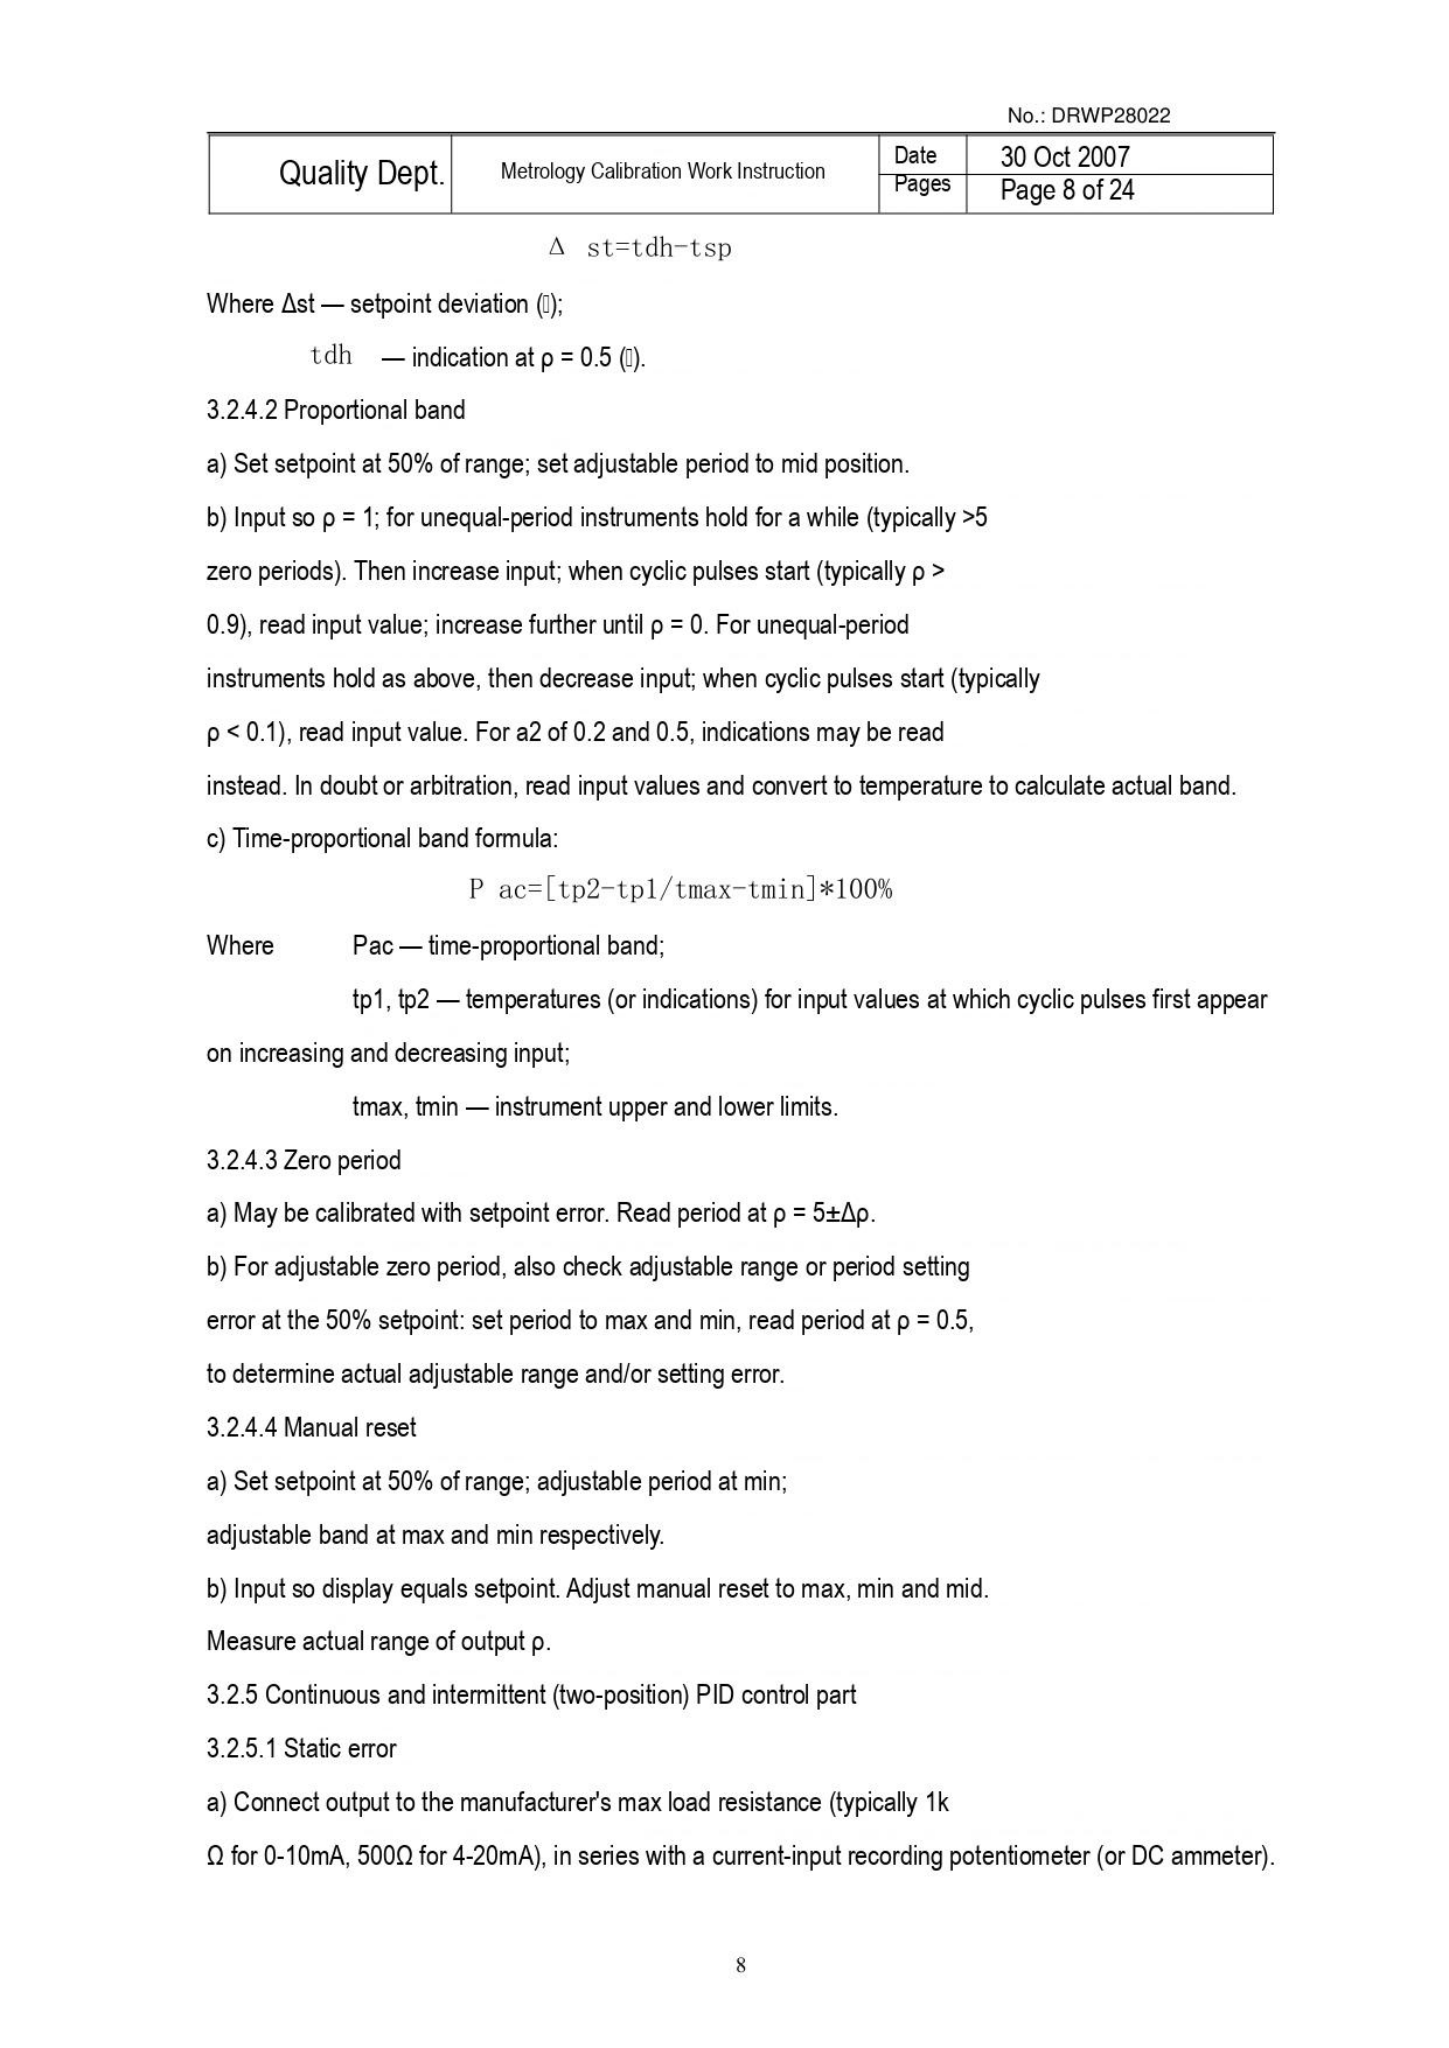No.: DRWP28022

| Quality Dept. | Metrology Calibration Work Instruction | Date | 30 Oct 2007 |
|---|---|---|---|
| | | Pages | Page 8 of 24 |

Δ st=tdh-tsp

Where Δst — setpoint deviation ();

tdh — indication at ρ = 0.5 ().

3.2.4.2 Proportional band

a) Set setpoint at 50% of range; set adjustable period to mid position.

b) Input so ρ = 1; for unequal-period instruments hold for a while (typically >5 zero periods). Then increase input; when cyclic pulses start (typically ρ > 0.9), read input value; increase further until ρ = 0. For unequal-period instruments hold as above, then decrease input; when cyclic pulses start (typically ρ < 0.1), read input value. For a2 of 0.2 and 0.5, indications may be read instead. In doubt or arbitration, read input values and convert to temperature to calculate actual band.

c) Time-proportional band formula:

P ac=[tp2-tp1/tmax-tmin]*100%

Where Pac — time-proportional band;

tp1, tp2 — temperatures (or indications) for input values at which cyclic pulses first appear on increasing and decreasing input;

tmax, tmin — instrument upper and lower limits.

3.2.4.3 Zero period

a) May be calibrated with setpoint error. Read period at ρ = 5±Δρ.

b) For adjustable zero period, also check adjustable range or period setting error at the 50% setpoint: set period to max and min, read period at ρ = 0.5, to determine actual adjustable range and/or setting error.

3.2.4.4 Manual reset

a) Set setpoint at 50% of range; adjustable period at min; adjustable band at max and min respectively.

b) Input so display equals setpoint. Adjust manual reset to max, min and mid. Measure actual range of output ρ.

3.2.5 Continuous and intermittent (two-position) PID control part

3.2.5.1 Static error

a) Connect output to the manufacturer's max load resistance (typically 1k Ω for 0-10mA, 500Ω for 4-20mA), in series with a current-input recording potentiometer (or DC ammeter).

8
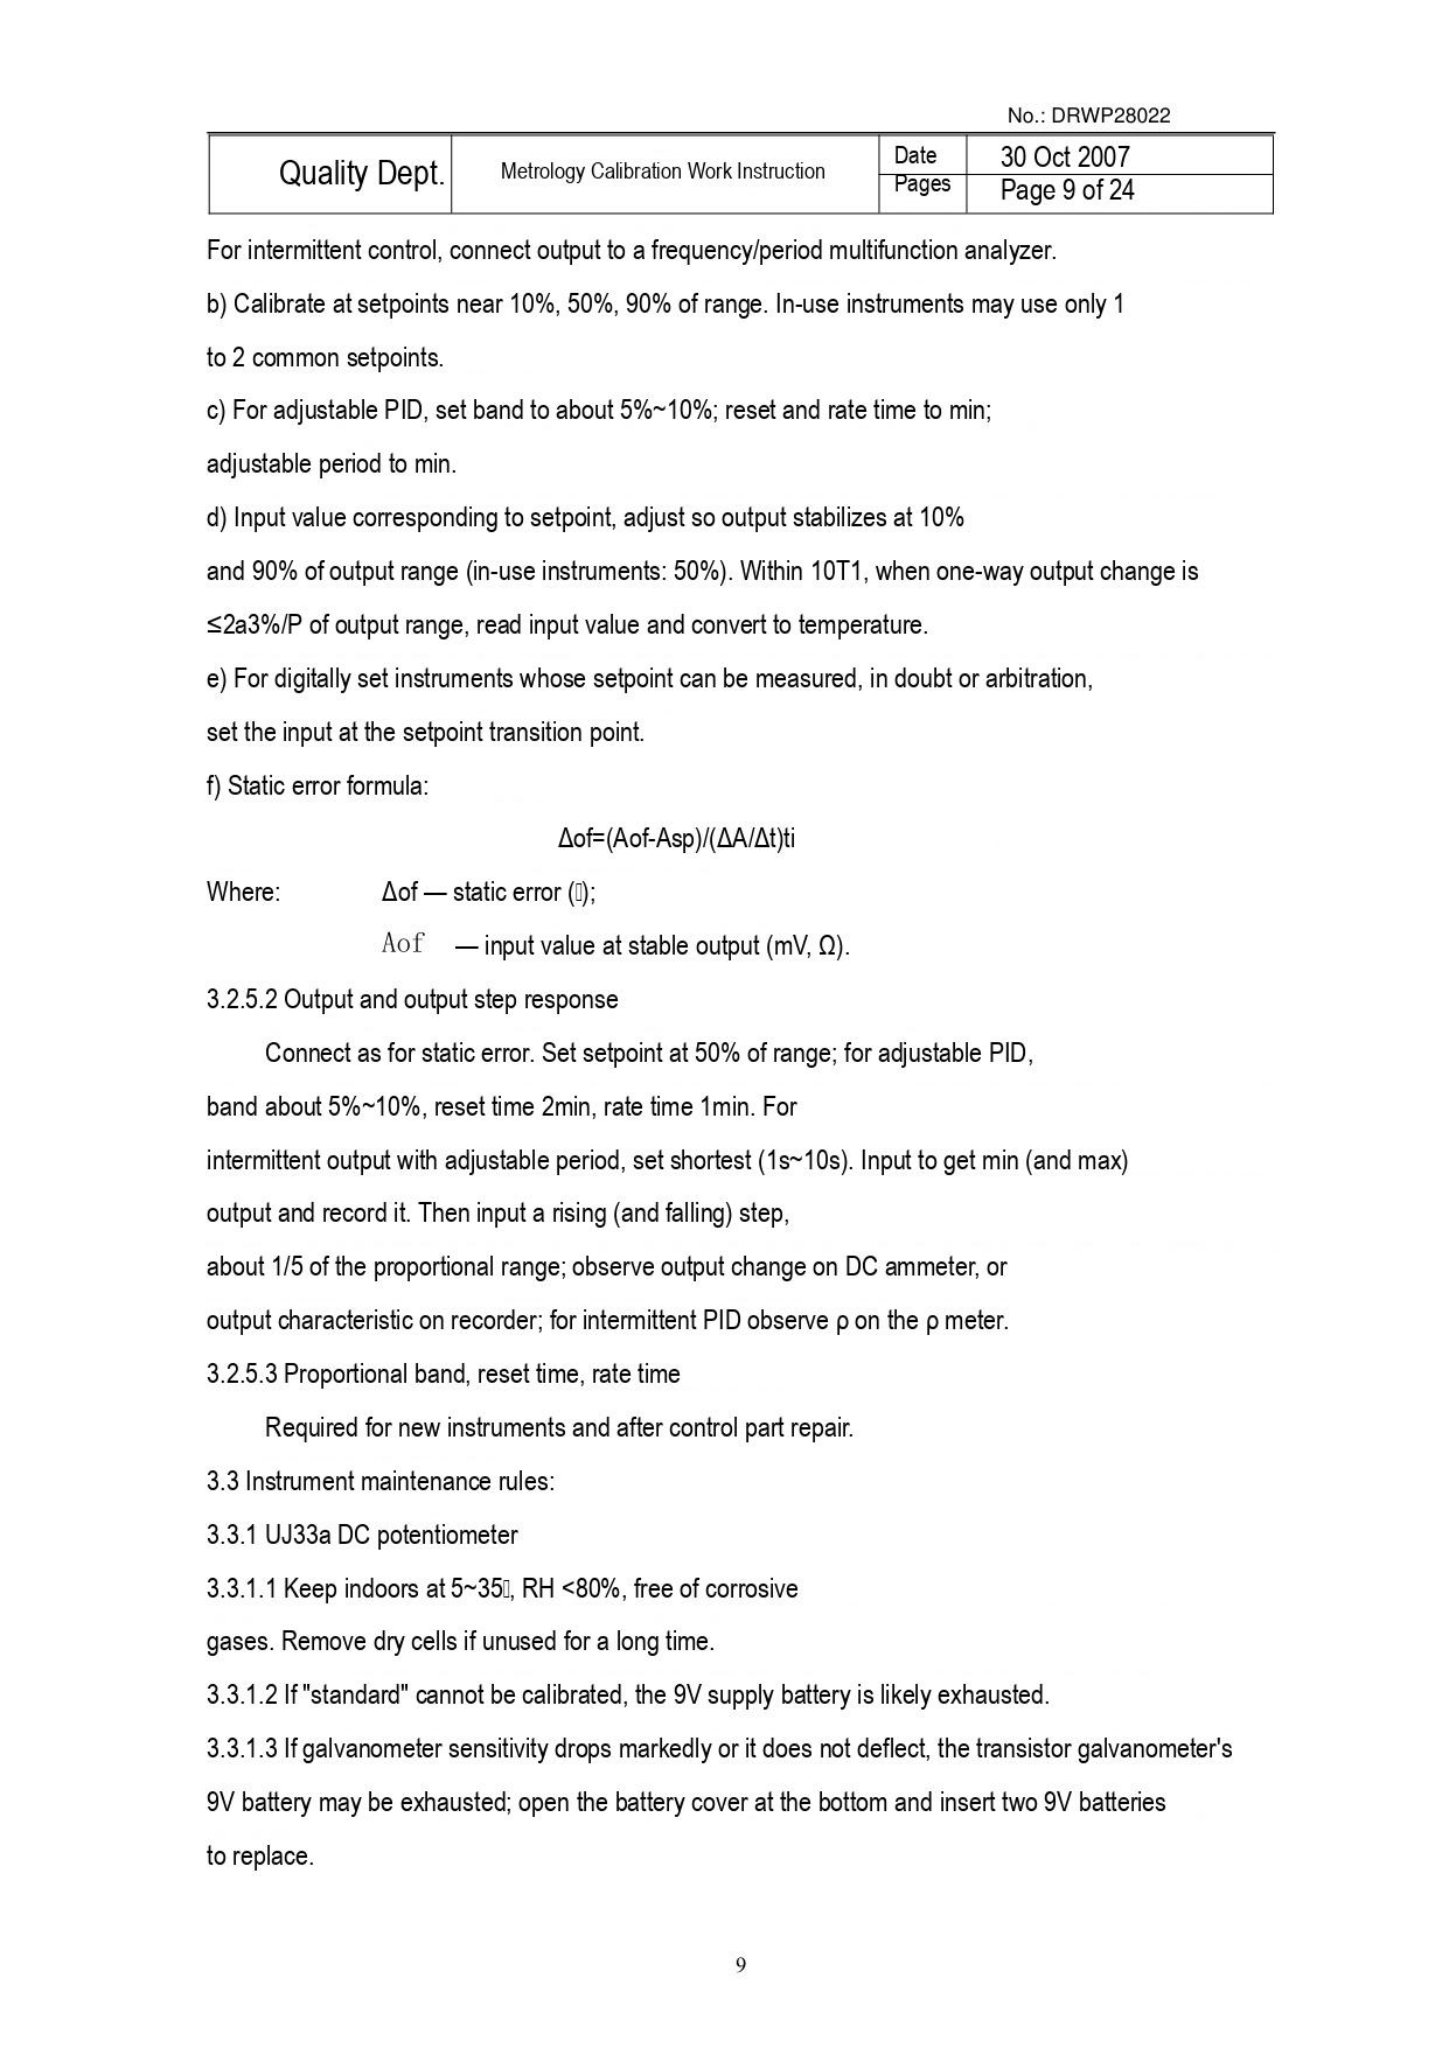No.: DRWP28022

| Quality Dept. | Metrology Calibration Work Instruction | Date | 30 Oct 2007 |
|---|---|---|---|
| | | Pages | Page 9 of 24 |

For intermittent control, connect output to a frequency/period multifunction analyzer.

b) Calibrate at setpoints near 10%, 50%, 90% of range. In-use instruments may use only 1 to 2 common setpoints.

c) For adjustable PID, set band to about 5%~10%; reset and rate time to min; adjustable period to min.

d) Input value corresponding to setpoint, adjust so output stabilizes at 10% and 90% of output range (in-use instruments: 50%). Within 10T1, when one-way output change is ≤2a3%/P of output range, read input value and convert to temperature.

e) For digitally set instruments whose setpoint can be measured, in doubt or arbitration, set the input at the setpoint transition point.

f) Static error formula:

Δof=(Aof-Asp)/(ΔA/Δt)ti

Where: Δof — static error ();

Aof — input value at stable output (mV, Ω).

3.2.5.2 Output and output step response

Connect as for static error. Set setpoint at 50% of range; for adjustable PID, band about 5%~10%, reset time 2min, rate time 1min. For intermittent output with adjustable period, set shortest (1s~10s). Input to get min (and max) output and record it. Then input a rising (and falling) step, about 1/5 of the proportional range; observe output change on DC ammeter, or output characteristic on recorder; for intermittent PID observe ρ on the ρ meter.

3.2.5.3 Proportional band, reset time, rate time

Required for new instruments and after control part repair.

3.3 Instrument maintenance rules:

3.3.1 UJ33a DC potentiometer

3.3.1.1 Keep indoors at 5~35, RH <80%, free of corrosive gases. Remove dry cells if unused for a long time.

3.3.1.2 If "standard" cannot be calibrated, the 9V supply battery is likely exhausted.

3.3.1.3 If galvanometer sensitivity drops markedly or it does not deflect, the transistor galvanometer's 9V battery may be exhausted; open the battery cover at the bottom and insert two 9V batteries to replace.

9
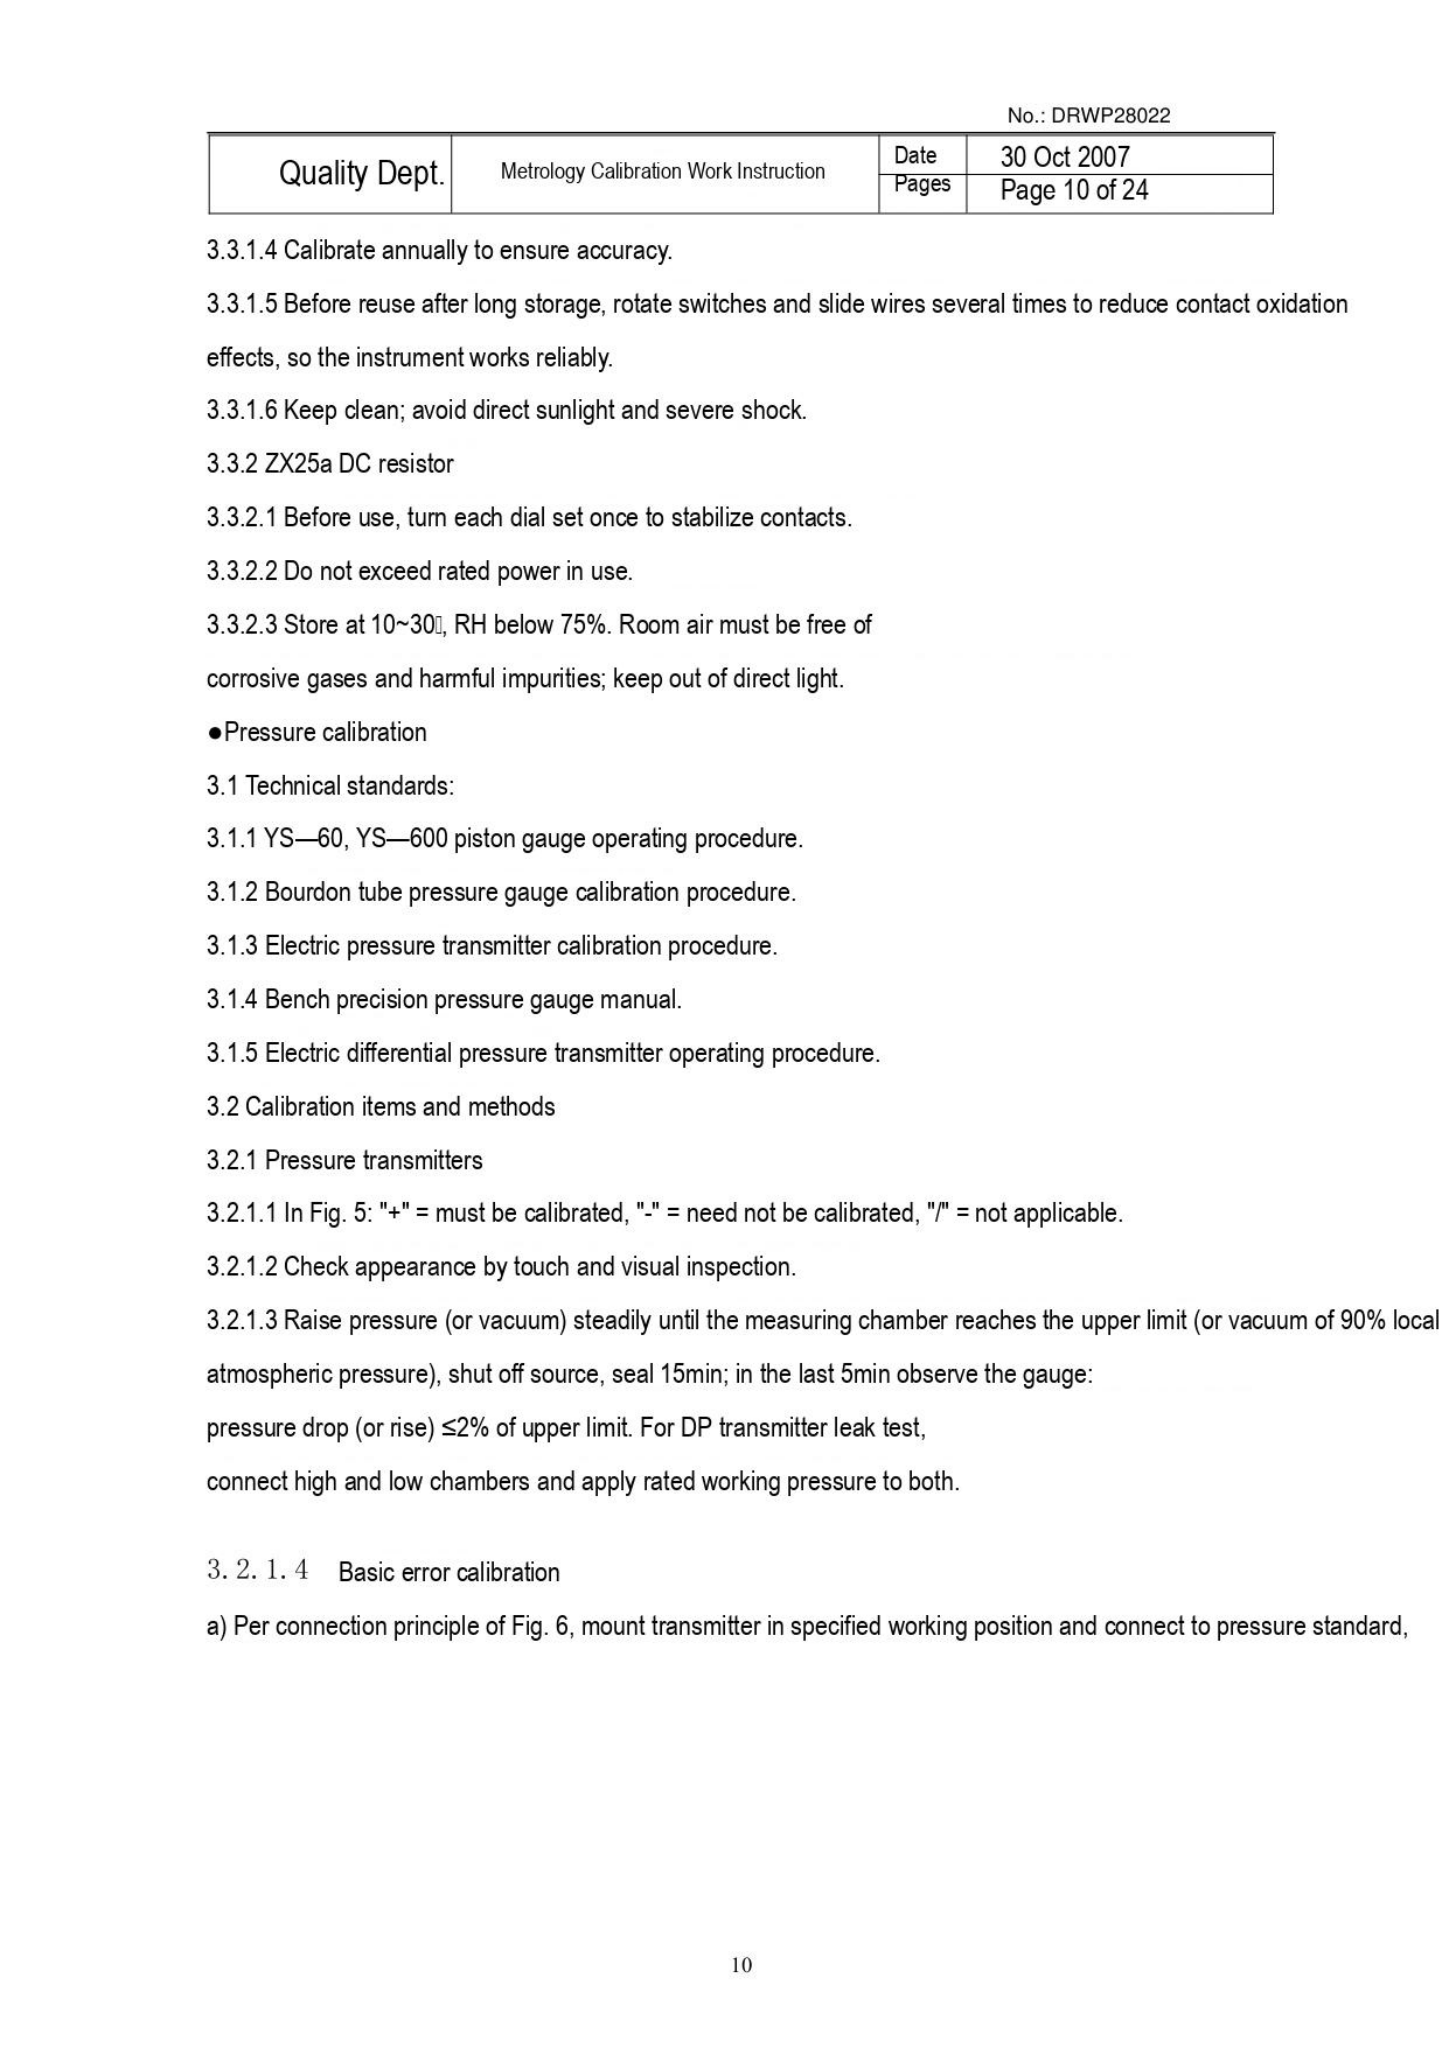No.: DRWP28022

| Quality Dept. | Metrology Calibration Work Instruction | Date | 30 Oct 2007 |
|---|---|---|---|
| | | Pages | Page 10 of 24 |

3.3.1.4 Calibrate annually to ensure accuracy.

3.3.1.5 Before reuse after long storage, rotate switches and slide wires several times to reduce contact oxidation effects, so the instrument works reliably.

3.3.1.6 Keep clean; avoid direct sunlight and severe shock.

3.3.2 ZX25a DC resistor

3.3.2.1 Before use, turn each dial set once to stabilize contacts.

3.3.2.2 Do not exceed rated power in use.

3.3.2.3 Store at 10~30, RH below 75%. Room air must be free of corrosive gases and harmful impurities; keep out of direct light.

●Pressure calibration

3.1 Technical standards:

3.1.1 YS—60, YS—600 piston gauge operating procedure.

3.1.2 Bourdon tube pressure gauge calibration procedure.

3.1.3 Electric pressure transmitter calibration procedure.

3.1.4 Bench precision pressure gauge manual.

3.1.5 Electric differential pressure transmitter operating procedure.

3.2 Calibration items and methods

3.2.1 Pressure transmitters

3.2.1.1 In Fig. 5: "+" = must be calibrated, "-" = need not be calibrated, "/" = not applicable.

3.2.1.2 Check appearance by touch and visual inspection.

3.2.1.3 Raise pressure (or vacuum) steadily until the measuring chamber reaches the upper limit (or vacuum of 90% local atmospheric pressure), shut off source, seal 15min; in the last 5min observe the gauge: pressure drop (or rise) ≤2% of upper limit. For DP transmitter leak test, connect high and low chambers and apply rated working pressure to both.

3.2.1.4 Basic error calibration

a) Per connection principle of Fig. 6, mount transmitter in specified working position and connect to pressure standard,

10
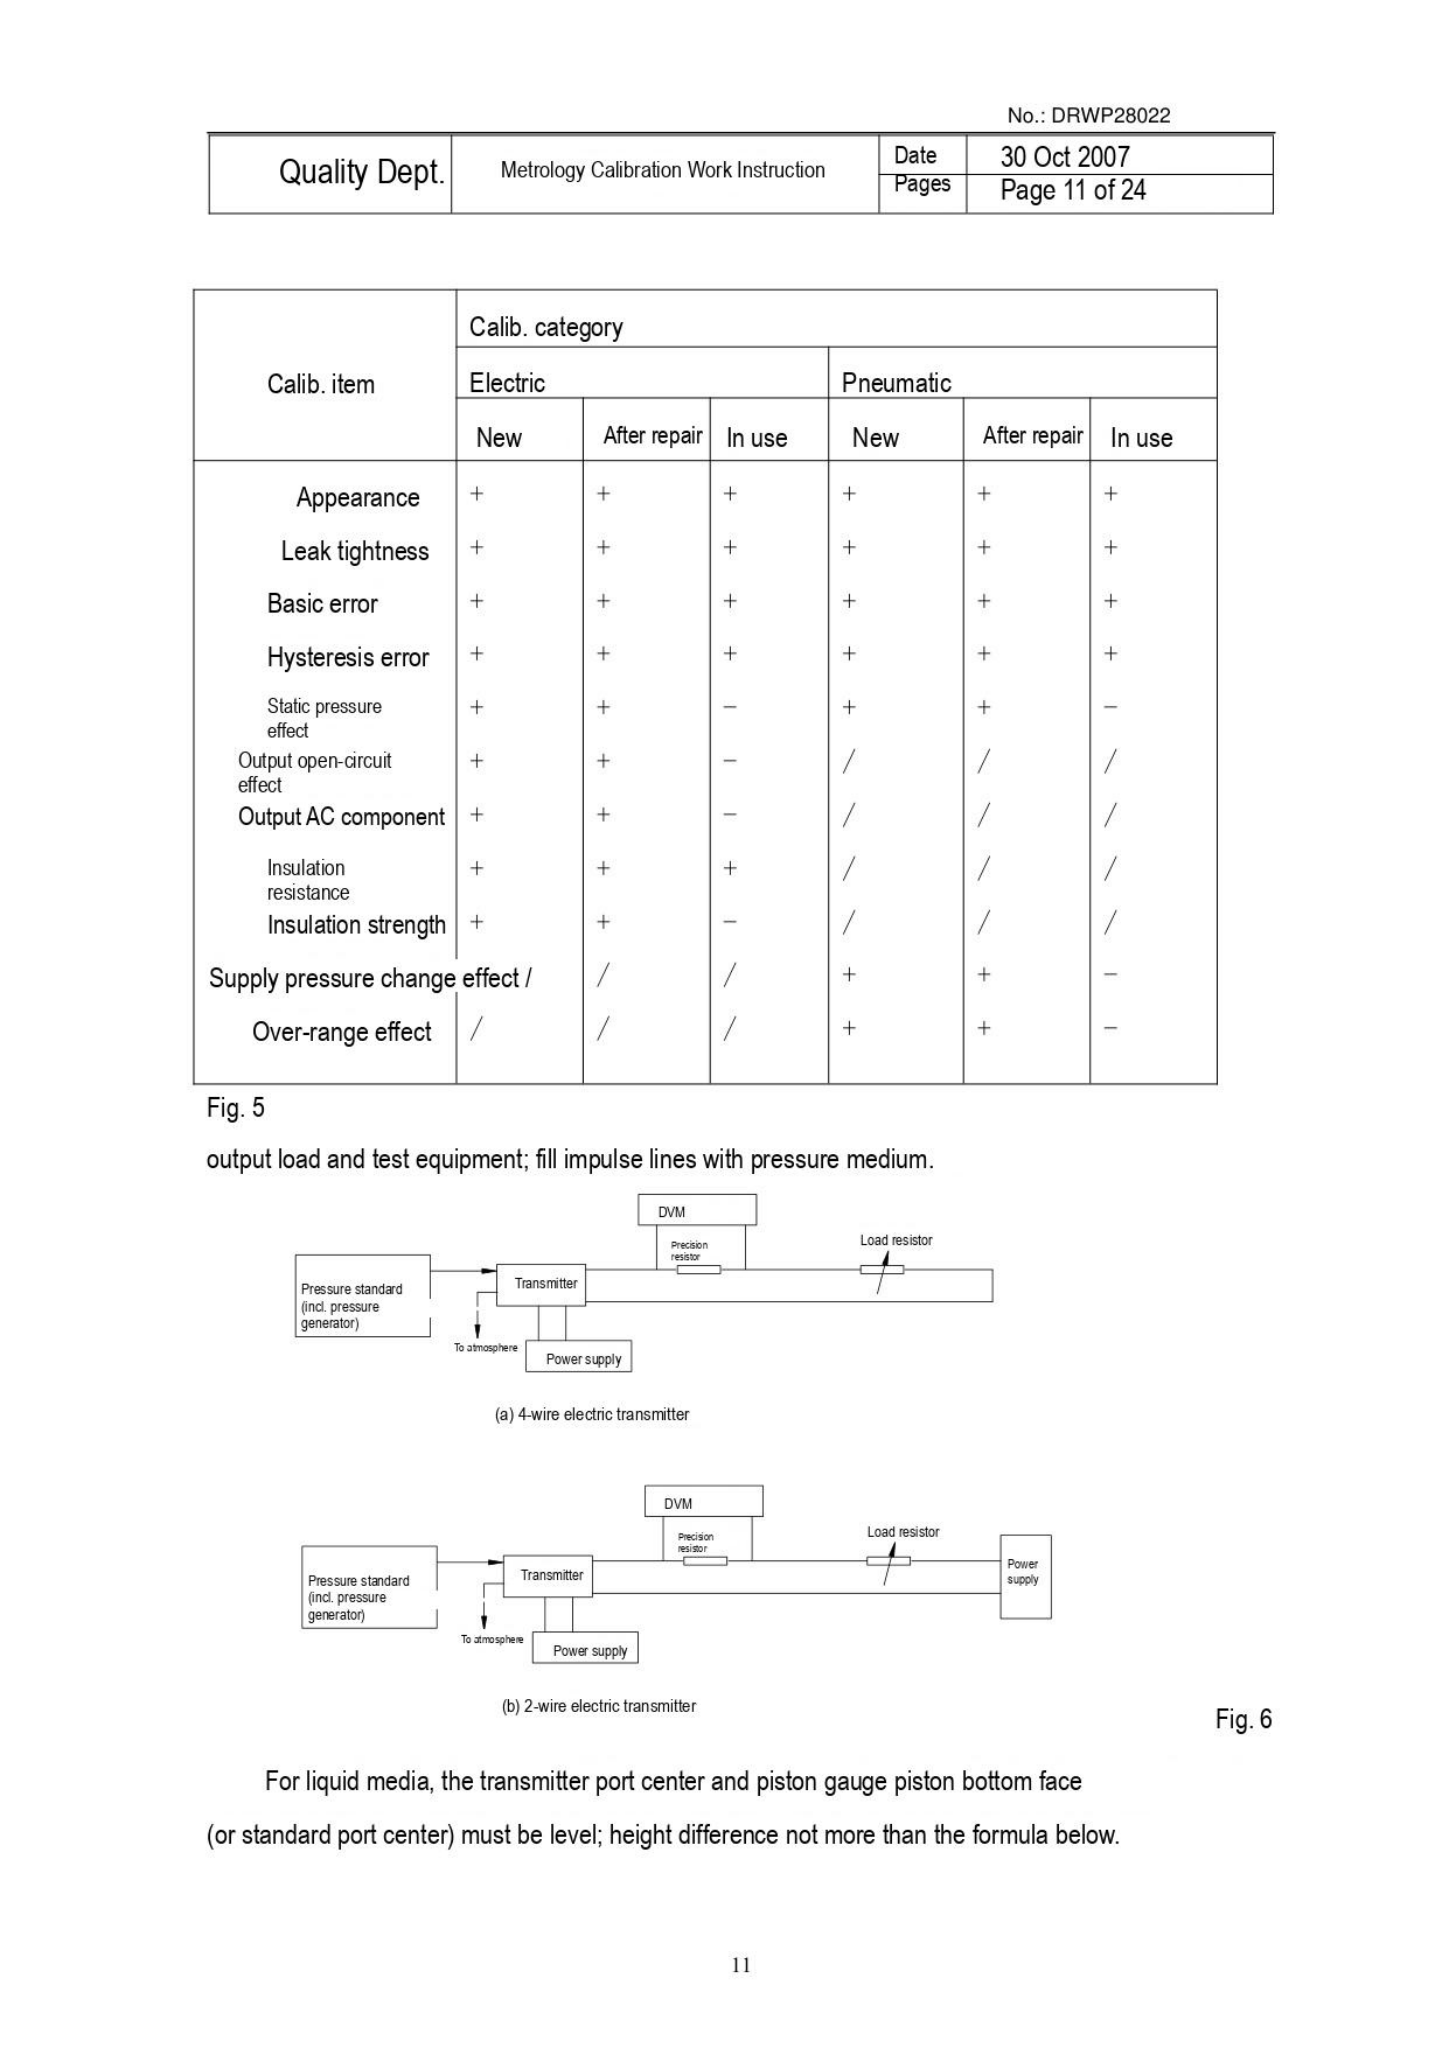No.: DRWP28022

| Quality Dept. | Metrology Calibration Work Instruction | Date | 30 Oct 2007 |
|---|---|---|---|
| | | Pages | Page 11 of 24 |

| Calib. item | Calib. category | | | | | |
|---|---|---|---|---|---|---|
| | Electric | | | Pneumatic | | |
| | New | After repair | In use | New | After repair | In use |
| Appearance | + | + | + | + | + | + |
| Leak tightness | + | + | + | + | + | + |
| Basic error | + | + | + | + | + | + |
| Hysteresis error | + | + | + | + | + | + |
| Static pressure effect | + | + | − | + | + | − |
| Output open-circuit effect | + | + | − | / | / | / |
| Output AC component | + | + | − | / | / | / |
| Insulation resistance | + | + | + | / | / | / |
| Insulation strength | + | + | − | / | / | / |
| Supply pressure change effect | / | / | / | + | + | − |
| Over-range effect | / | / | / | + | + | − |

Fig. 5

output load and test equipment; fill impulse lines with pressure medium.

DVM
Precision resistor
Load resistor
Pressure standard (incl. pressure generator)
Transmitter
To atmosphere
Power supply

(a) 4-wire electric transmitter

DVM
Precision resistor
Load resistor
Power supply
Pressure standard (incl. pressure generator)
Transmitter
To atmosphere
Power supply

(b) 2-wire electric transmitter

Fig. 6

For liquid media, the transmitter port center and piston gauge piston bottom face (or standard port center) must be level; height difference not more than the formula below.

11
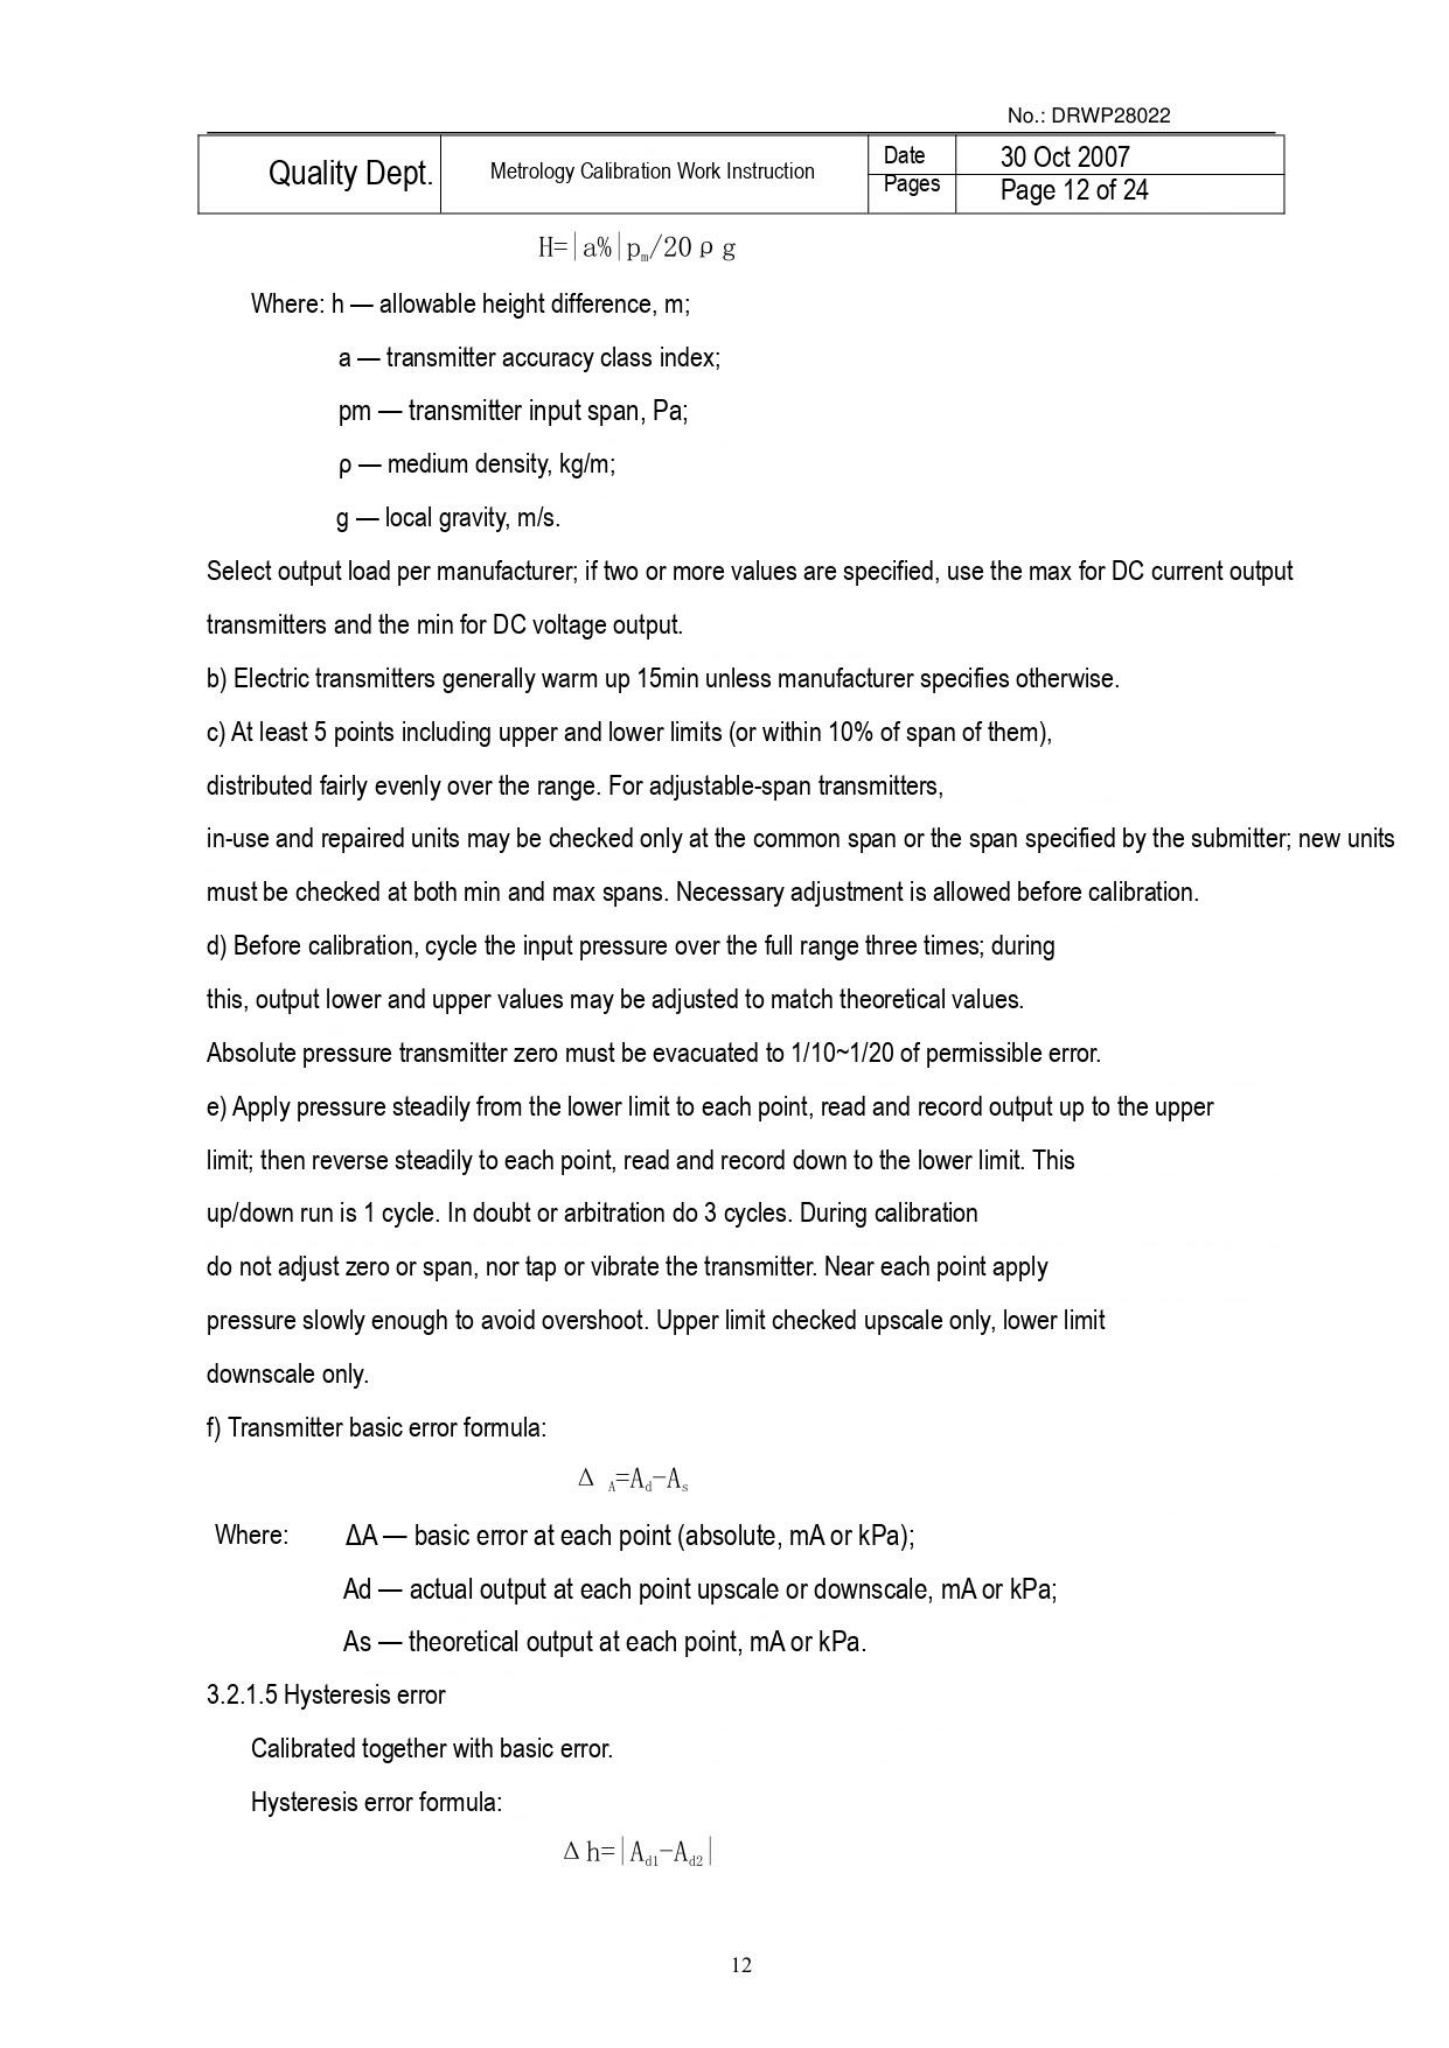No.: DRWP28022

| Quality Dept. | Metrology Calibration Work Instruction | Date | 30 Oct 2007 |
|---|---|---|---|
| | | Pages | Page 12 of 24 |

H=|a%|p<sub>m</sub>/20ρg

Where: h — allowable height difference, m;

a — transmitter accuracy class index;

pm — transmitter input span, Pa;

ρ — medium density, kg/m;

g — local gravity, m/s.

Select output load per manufacturer; if two or more values are specified, use the max for DC current output transmitters and the min for DC voltage output.

b) Electric transmitters generally warm up 15min unless manufacturer specifies otherwise.

c) At least 5 points including upper and lower limits (or within 10% of span of them), distributed fairly evenly over the range. For adjustable-span transmitters, in-use and repaired units may be checked only at the common span or the span specified by the submitter; new units must be checked at both min and max spans. Necessary adjustment is allowed before calibration.

d) Before calibration, cycle the input pressure over the full range three times; during this, output lower and upper values may be adjusted to match theoretical values. Absolute pressure transmitter zero must be evacuated to 1/10~1/20 of permissible error.

e) Apply pressure steadily from the lower limit to each point, read and record output up to the upper limit; then reverse steadily to each point, read and record down to the lower limit. This up/down run is 1 cycle. In doubt or arbitration do 3 cycles. During calibration do not adjust zero or span, nor tap or vibrate the transmitter. Near each point apply pressure slowly enough to avoid overshoot. Upper limit checked upscale only, lower limit downscale only.

f) Transmitter basic error formula:

Δ<sub>A</sub>=A<sub>d</sub>−A<sub>s</sub>

Where: ΔA — basic error at each point (absolute, mA or kPa);

Ad — actual output at each point upscale or downscale, mA or kPa;

As — theoretical output at each point, mA or kPa.

3.2.1.5 Hysteresis error

Calibrated together with basic error.

Hysteresis error formula:

Δh=|A<sub>d1</sub>−A<sub>d2</sub>|

12
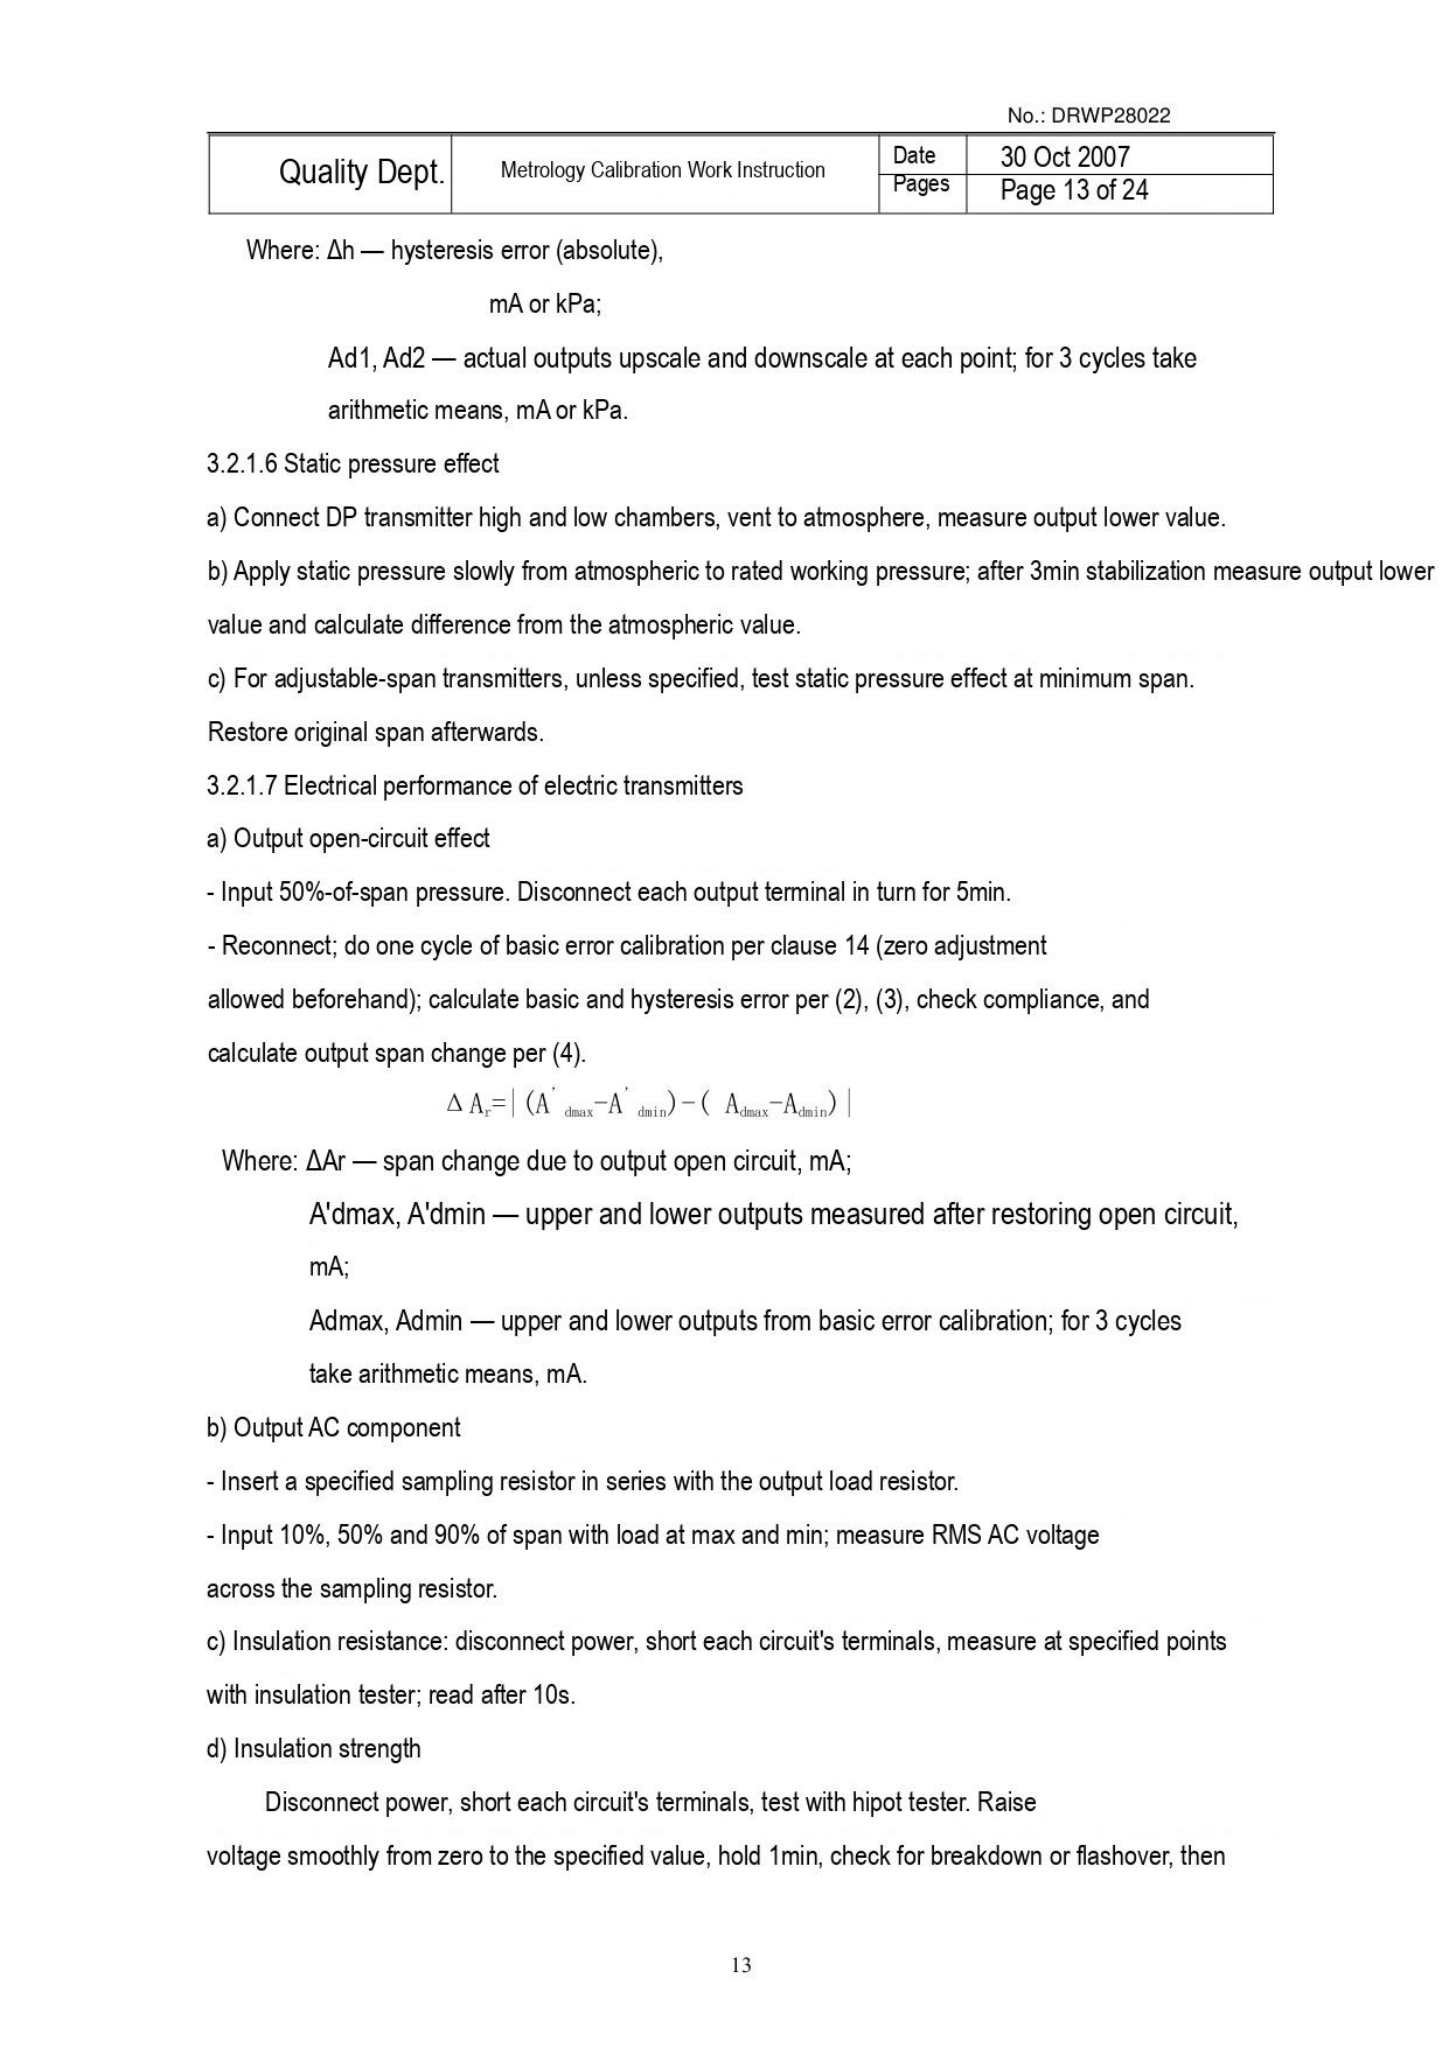No.: DRWP28022

| Quality Dept. | Metrology Calibration Work Instruction | Date | 30 Oct 2007 |
|---|---|---|---|
| | | Pages | Page 13 of 24 |

Where: Δh — hysteresis error (absolute),

mA or kPa;

Ad1, Ad2 — actual outputs upscale and downscale at each point; for 3 cycles take arithmetic means, mA or kPa.

3.2.1.6 Static pressure effect

a) Connect DP transmitter high and low chambers, vent to atmosphere, measure output lower value.

b) Apply static pressure slowly from atmospheric to rated working pressure; after 3min stabilization measure output lower value and calculate difference from the atmospheric value.

c) For adjustable-span transmitters, unless specified, test static pressure effect at minimum span. Restore original span afterwards.

3.2.1.7 Electrical performance of electric transmitters

a) Output open-circuit effect

- Input 50%-of-span pressure. Disconnect each output terminal in turn for 5min.

- Reconnect; do one cycle of basic error calibration per clause 14 (zero adjustment allowed beforehand); calculate basic and hysteresis error per (2), (3), check compliance, and calculate output span change per (4).

ΔA<sub>r</sub>=|(A'<sub>dmax</sub>−A'<sub>dmin</sub>)−(A<sub>dmax</sub>−A<sub>dmin</sub>)|

Where: ΔAr — span change due to output open circuit, mA;

A'dmax, A'dmin — upper and lower outputs measured after restoring open circuit, mA;

Admax, Admin — upper and lower outputs from basic error calibration; for 3 cycles take arithmetic means, mA.

b) Output AC component

- Insert a specified sampling resistor in series with the output load resistor.

- Input 10%, 50% and 90% of span with load at max and min; measure RMS AC voltage across the sampling resistor.

c) Insulation resistance: disconnect power, short each circuit's terminals, measure at specified points with insulation tester; read after 10s.

d) Insulation strength

Disconnect power, short each circuit's terminals, test with hipot tester. Raise voltage smoothly from zero to the specified value, hold 1min, check for breakdown or flashover, then

13